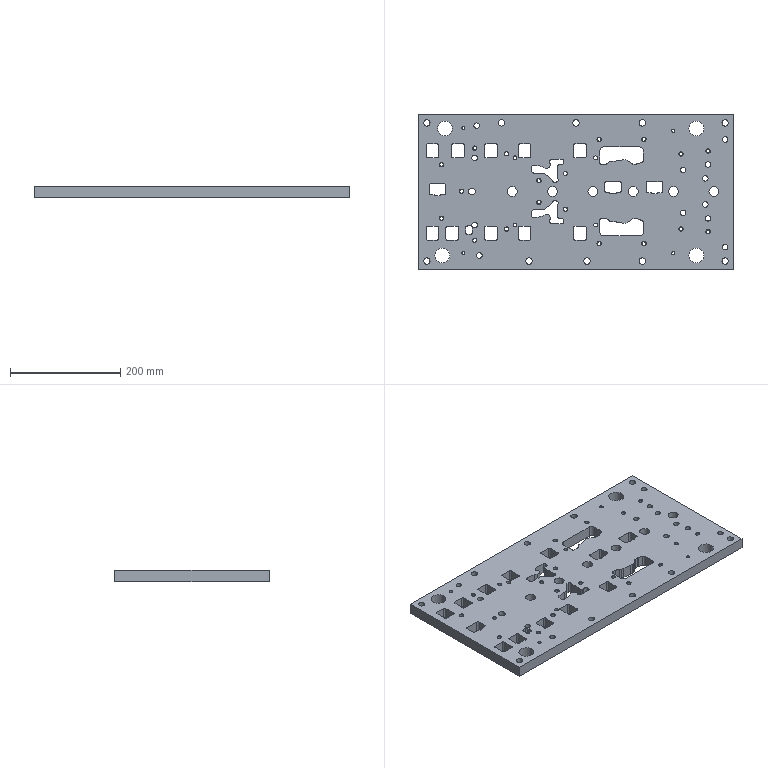Part | NX | features LB-3 2 | 1 solid | 315 faces | box 570 x 280 x 20 mm | volume 2769913 mm3 | cylinder 140 | plane 108 | spline 44 | cone 23 | commonest cylinder face diameters 5 x40 6.8 x18 6 x14 1 x12 10 x10 11.5 x10